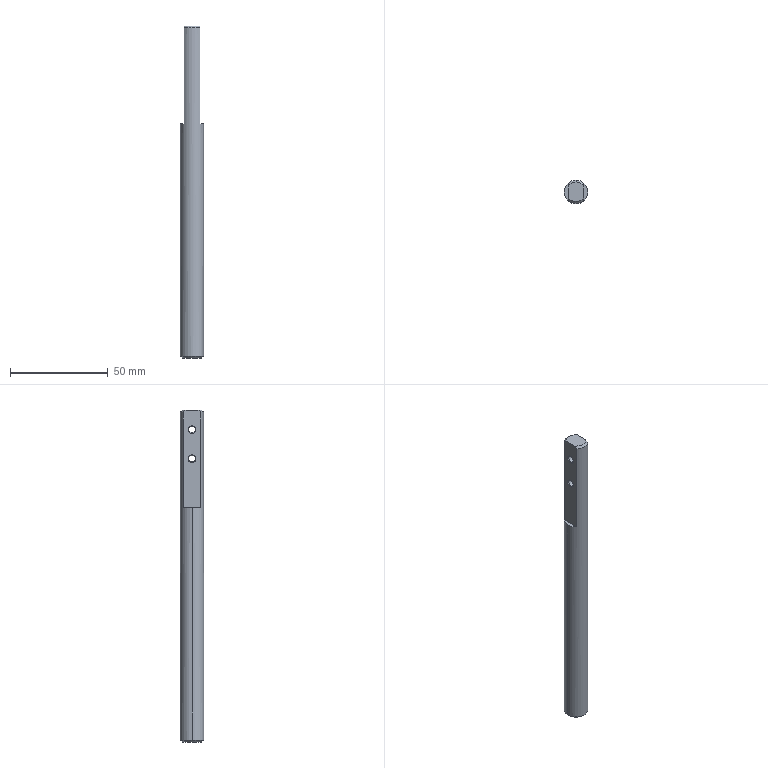Part | SolidWorks | features Chamfer 1, Extrusion 1, HoleWzd 1, ICE 1 | 1 solid | 20 faces | box 12 x 12 x 170 mm | volume 17822 mm3 | cone 8 | cylinder 6 | plane 6 | commonest cylinder face diameters 3.3 x4 12 x2
STEP:
#1=CARTESIAN_POINT('',(-3.625,0.,158.35));
#2=VERTEX_POINT('',#1);
#3=CARTESIAN_POINT('',(-3.625,0.,161.65));
#4=VERTEX_POINT('',#3);
#5=CARTESIAN_POINT('',(-3.625,0.,160.));
#6=DIRECTION('',(-1.,0.,0.));
#7=DIRECTION('',(0.,0.,1.));
#8=AXIS2_PLACEMENT_3D('',#5,#6,#7);
#9=CIRCLE('',#8,1.65);
#10=EDGE_CURVE('',#2,#4,#9,.T.);
#11=ORIENTED_EDGE('',*,*,#10,.F.);
#12=CARTESIAN_POINT('',(-4.,0.,157.975));
#13=VERTEX_POINT('',#12);
#14=CARTESIAN_POINT('',(-4.,0.,157.975));
#15=DIRECTION('',(-0.7071,0.,-0.7071));
#16=VECTOR('',#15,1000.);
#17=LINE('',#14,#16);
#18=EDGE_CURVE('',#2,#13,#17,.T.);
#19=ORIENTED_EDGE('',*,*,#18,.T.);
#20=CARTESIAN_POINT('',(-4.,0.,162.025));
#21=VERTEX_POINT('',#20);
#22=CARTESIAN_POINT('',(-4.,0.,160.));
#23=DIRECTION('',(-1.,0.,0.));
#24=DIRECTION('',(0.,0.,1.));
#25=AXIS2_PLACEMENT_3D('',#22,#23,#24);
#26=CIRCLE('',#25,2.025);
#27=EDGE_CURVE('',#13,#21,#26,.T.);
#28=ORIENTED_EDGE('',*,*,#27,.T.);
#29=CARTESIAN_POINT('',(-4.,0.,162.025));
#30=DIRECTION('',(-0.7071,0.,0.7071));
#31=VECTOR('',#30,1000.);
#32=LINE('',#29,#31);
#33=EDGE_CURVE('',#4,#21,#32,.T.);
#34=ORIENTED_EDGE('',*,*,#33,.F.);
#35=EDGE_LOOP('',(#11,#19,#28,#34));
#36=FACE_OUTER_BOUND('',#35,.T.);
#37=CARTESIAN_POINT('',(-4.,0.,160.));
#38=DIRECTION('',(-1.,0.,0.));
#39=DIRECTION('',(0.,0.,1.));
#40=AXIS2_PLACEMENT_3D('',#37,#38,#39);
#41=CONICAL_SURFACE('',#40,2.025,0.7854);
#42=ADVANCED_FACE('',(#36),#41,.F.);
#43=CARTESIAN_POINT('',(4.,0.,158.35));
#44=VERTEX_POINT('',#43);
#45=CARTESIAN_POINT('',(4.,0.,161.65));
#46=VERTEX_POINT('',#45);
#47=CARTESIAN_POINT('',(4.,0.,160.));
#48=DIRECTION('',(-1.,0.,0.));
#49=DIRECTION('',(0.,0.,1.));
#50=AXIS2_PLACEMENT_3D('',#47,#48,#49);
#51=CIRCLE('',#50,1.65);
#52=EDGE_CURVE('',#44,#46,#51,.T.);
#53=ORIENTED_EDGE('',*,*,#52,.F.);
#54=CARTESIAN_POINT('',(-4.,0.,158.35));
#55=DIRECTION('',(-1.,0.,0.));
#56=VECTOR('',#55,1000.);
#57=LINE('',#54,#56);
#58=EDGE_CURVE('',#44,#2,#57,.T.);
#59=ORIENTED_EDGE('',*,*,#58,.T.);
#60=ORIENTED_EDGE('',*,*,#10,.T.);
#61=CARTESIAN_POINT('',(-4.,0.,161.65));
#62=DIRECTION('',(-1.,0.,0.));
#63=VECTOR('',#62,1000.);
#64=LINE('',#61,#63);
#65=EDGE_CURVE('',#46,#4,#64,.T.);
#66=ORIENTED_EDGE('',*,*,#65,.F.);
#67=EDGE_LOOP('',(#53,#59,#60,#66));
#68=FACE_OUTER_BOUND('',#67,.T.);
#69=CARTESIAN_POINT('',(-4.,0.,160.));
#70=DIRECTION('',(-1.,0.,0.));
#71=DIRECTION('',(0.,0.,1.));
#72=AXIS2_PLACEMENT_3D('',#69,#70,#71);
#73=CYLINDRICAL_SURFACE('',#72,1.65);
#74=ADVANCED_FACE('',(#68),#73,.F.);
#75=CARTESIAN_POINT('',(-3.625,0.,143.35));
#76=VERTEX_POINT('',#75);
#77=CARTESIAN_POINT('',(-3.625,0.,146.65));
#78=VERTEX_POINT('',#77);
#79=CARTESIAN_POINT('',(-3.625,0.,145.));
#80=DIRECTION('',(-1.,0.,0.));
#81=DIRECTION('',(0.,0.,1.));
#82=AXIS2_PLACEMENT_3D('',#79,#80,#81);
#83=CIRCLE('',#82,1.65);
#84=EDGE_CURVE('',#76,#78,#83,.T.);
#85=ORIENTED_EDGE('',*,*,#84,.F.);
#86=CARTESIAN_POINT('',(-4.,0.,142.975));
#87=VERTEX_POINT('',#86);
#88=CARTESIAN_POINT('',(-4.,0.,142.975));
#89=DIRECTION('',(-0.7071,0.,-0.7071));
#90=VECTOR('',#89,1000.);
#91=LINE('',#88,#90);
#92=EDGE_CURVE('',#76,#87,#91,.T.);
#93=ORIENTED_EDGE('',*,*,#92,.T.);
#94=CARTESIAN_POINT('',(-4.,0.,147.025));
#95=VERTEX_POINT('',#94);
#96=CARTESIAN_POINT('',(-4.,0.,145.));
#97=DIRECTION('',(-1.,0.,0.));
#98=DIRECTION('',(0.,0.,1.));
#99=AXIS2_PLACEMENT_3D('',#96,#97,#98);
#100=CIRCLE('',#99,2.025);
#101=EDGE_CURVE('',#87,#95,#100,.T.);
#102=ORIENTED_EDGE('',*,*,#101,.T.);
#103=CARTESIAN_POINT('',(-4.,0.,147.025));
#104=DIRECTION('',(-0.7071,0.,0.7071));
#105=VECTOR('',#104,1000.);
#106=LINE('',#103,#105);
#107=EDGE_CURVE('',#78,#95,#106,.T.);
#108=ORIENTED_EDGE('',*,*,#107,.F.);
#109=EDGE_LOOP('',(#85,#93,#102,#108));
#110=FACE_OUTER_BOUND('',#109,.T.);
#111=CARTESIAN_POINT('',(-4.,0.,145.));
#112=DIRECTION('',(-1.,0.,0.));
#113=DIRECTION('',(0.,0.,1.));
#114=AXIS2_PLACEMENT_3D('',#111,#112,#113);
#115=CONICAL_SURFACE('',#114,2.025,0.7854);
#116=ADVANCED_FACE('',(#110),#115,.F.);
#117=CARTESIAN_POINT('',(4.,0.,143.35));
#118=VERTEX_POINT('',#117);
#119=CARTESIAN_POINT('',(4.,0.,146.65));
#120=VERTEX_POINT('',#119);
#121=CARTESIAN_POINT('',(4.,0.,145.));
#122=DIRECTION('',(-1.,0.,0.));
#123=DIRECTION('',(0.,0.,1.));
#124=AXIS2_PLACEMENT_3D('',#121,#122,#123);
#125=CIRCLE('',#124,1.65);
#126=EDGE_CURVE('',#118,#120,#125,.T.);
#127=ORIENTED_EDGE('',*,*,#126,.F.);
#128=CARTESIAN_POINT('',(-4.,0.,143.35));
#129=DIRECTION('',(-1.,0.,0.));
#130=VECTOR('',#129,1000.);
#131=LINE('',#128,#130);
#132=EDGE_CURVE('',#118,#76,#131,.T.);
#133=ORIENTED_EDGE('',*,*,#132,.T.);
#134=ORIENTED_EDGE('',*,*,#84,.T.);
#135=CARTESIAN_POINT('',(-4.,0.,146.65));
#136=DIRECTION('',(-1.,0.,0.));
#137=VECTOR('',#136,1000.);
#138=LINE('',#135,#137);
#139=EDGE_CURVE('',#120,#78,#138,.T.);
#140=ORIENTED_EDGE('',*,*,#139,.F.);
#141=EDGE_LOOP('',(#127,#133,#134,#140));
#142=FACE_OUTER_BOUND('',#141,.T.);
#143=CARTESIAN_POINT('',(-4.,0.,145.));
#144=DIRECTION('',(-1.,0.,0.));
#145=DIRECTION('',(0.,0.,1.));
#146=AXIS2_PLACEMENT_3D('',#143,#144,#145);
#147=CYLINDRICAL_SURFACE('',#146,1.65);
#148=ADVANCED_FACE('',(#142),#147,.F.);
#149=CARTESIAN_POINT('',(-5.,0.,0.));
#150=VERTEX_POINT('',#149);
#151=CARTESIAN_POINT('',(5.,0.,0.));
#152=VERTEX_POINT('',#151);
#153=CARTESIAN_POINT('',(0.,0.,0.));
#154=DIRECTION('',(0.,0.,-1.));
#155=DIRECTION('',(1.,0.,0.));
#156=AXIS2_PLACEMENT_3D('',#153,#154,#155);
#157=CIRCLE('',#156,5.);
#158=EDGE_CURVE('',#150,#152,#157,.T.);
#159=ORIENTED_EDGE('',*,*,#158,.F.);
#160=CARTESIAN_POINT('',(-6.,0.,1.));
#161=VERTEX_POINT('',#160);
#162=CARTESIAN_POINT('',(-6.,0.,1.));
#163=DIRECTION('',(-0.7071,0.,0.7071));
#164=VECTOR('',#163,1000.);
#165=LINE('',#162,#164);
#166=EDGE_CURVE('',#150,#161,#165,.T.);
#167=ORIENTED_EDGE('',*,*,#166,.T.);
#168=CARTESIAN_POINT('',(6.,0.,1.));
#169=VERTEX_POINT('',#168);
#170=CARTESIAN_POINT('',(0.,0.,1.));
#171=DIRECTION('',(0.,0.,1.));
#172=DIRECTION('',(1.,0.,0.));
#173=AXIS2_PLACEMENT_3D('',#170,#171,#172);
#174=CIRCLE('',#173,6.);
#175=EDGE_CURVE('',#169,#161,#174,.T.);
#176=ORIENTED_EDGE('',*,*,#175,.F.);
#177=CARTESIAN_POINT('',(6.,0.,1.));
#178=DIRECTION('',(0.7071,0.,0.7071));
#179=VECTOR('',#178,1000.);
#180=LINE('',#177,#179);
#181=EDGE_CURVE('',#152,#169,#180,.T.);
#182=ORIENTED_EDGE('',*,*,#181,.F.);
#183=EDGE_LOOP('',(#159,#167,#176,#182));
#184=FACE_OUTER_BOUND('',#183,.T.);
#185=CARTESIAN_POINT('',(0.,0.,1.));
#186=DIRECTION('',(0.,0.,1.));
#187=DIRECTION('',(1.,0.,0.));
#188=AXIS2_PLACEMENT_3D('',#185,#186,#187);
#189=CONICAL_SURFACE('',#188,6.,0.7854);
#190=ADVANCED_FACE('',(#184),#189,.T.);
#191=CARTESIAN_POINT('',(4.,4.472,120.));
#192=VERTEX_POINT('',#191);
#193=CARTESIAN_POINT('',(6.,0.,120.));
#194=VERTEX_POINT('',#193);
#195=CARTESIAN_POINT('',(0.,0.,120.));
#196=DIRECTION('',(0.,0.,-1.));
#197=DIRECTION('',(-1.,0.,0.));
#198=AXIS2_PLACEMENT_3D('',#195,#196,#197);
#199=CIRCLE('',#198,6.);
#200=EDGE_CURVE('',#192,#194,#199,.T.);
#201=ORIENTED_EDGE('',*,*,#200,.T.);
#202=CARTESIAN_POINT('',(6.,0.,170.));
#203=DIRECTION('',(0.,0.,-1.));
#204=VECTOR('',#203,1000.);
#205=LINE('',#202,#204);
#206=EDGE_CURVE('',#194,#169,#205,.T.);
#207=ORIENTED_EDGE('',*,*,#206,.T.);
#208=ORIENTED_EDGE('',*,*,#175,.T.);
#209=CARTESIAN_POINT('',(-6.,0.,120.));
#210=VERTEX_POINT('',#209);
#211=CARTESIAN_POINT('',(-6.,0.,170.));
#212=DIRECTION('',(0.,0.,-1.));
#213=VECTOR('',#212,1000.);
#214=LINE('',#211,#213);
#215=EDGE_CURVE('',#210,#161,#214,.T.);
#216=ORIENTED_EDGE('',*,*,#215,.F.);
#217=CARTESIAN_POINT('',(-4.,4.472,120.));
#218=VERTEX_POINT('',#217);
#219=CARTESIAN_POINT('',(0.,0.,120.));
#220=DIRECTION('',(0.,0.,-1.));
#221=DIRECTION('',(-1.,0.,0.));
#222=AXIS2_PLACEMENT_3D('',#219,#220,#221);
#223=CIRCLE('',#222,6.);
#224=EDGE_CURVE('',#210,#218,#223,.T.);
#225=ORIENTED_EDGE('',*,*,#224,.T.);
#226=CARTESIAN_POINT('',(-4.,4.472,169.));
#227=VERTEX_POINT('',#226);
#228=CARTESIAN_POINT('',(-4.,4.472,170.));
#229=DIRECTION('',(0.,0.,1.));
#230=VECTOR('',#229,1000.);
#231=LINE('',#228,#230);
#232=EDGE_CURVE('',#218,#227,#231,.T.);
#233=ORIENTED_EDGE('',*,*,#232,.T.);
#234=CARTESIAN_POINT('',(4.,4.472,169.));
#235=VERTEX_POINT('',#234);
#236=CARTESIAN_POINT('',(0.,0.,169.));
#237=DIRECTION('',(0.,0.,-1.));
#238=DIRECTION('',(1.,0.,0.));
#239=AXIS2_PLACEMENT_3D('',#236,#237,#238);
#240=CIRCLE('',#239,6.);
#241=EDGE_CURVE('',#227,#235,#240,.T.);
#242=ORIENTED_EDGE('',*,*,#241,.T.);
#243=CARTESIAN_POINT('',(4.,4.472,170.));
#244=DIRECTION('',(0.,0.,-1.));
#245=VECTOR('',#244,1000.);
#246=LINE('',#243,#245);
#247=EDGE_CURVE('',#235,#192,#246,.T.);
#248=ORIENTED_EDGE('',*,*,#247,.T.);
#249=EDGE_LOOP('',(#201,#207,#208,#216,#225,#233,#242,#248));
#250=FACE_OUTER_BOUND('',#249,.T.);
#251=CARTESIAN_POINT('',(0.,0.,170.));
#252=DIRECTION('',(0.,0.,-1.));
#253=DIRECTION('',(-1.,0.,0.));
#254=AXIS2_PLACEMENT_3D('',#251,#252,#253);
#255=CYLINDRICAL_SURFACE('',#254,6.);
#256=ADVANCED_FACE('',(#250),#255,.T.);
#257=CARTESIAN_POINT('',(-4.,0.,160.));
#258=DIRECTION('',(-1.,0.,0.));
#259=DIRECTION('',(0.,0.,1.));
#260=AXIS2_PLACEMENT_3D('',#257,#258,#259);
#261=CIRCLE('',#260,2.025);
#262=EDGE_CURVE('',#21,#13,#261,.T.);
#263=ORIENTED_EDGE('',*,*,#262,.F.);
#264=ORIENTED_EDGE('',*,*,#27,.F.);
#265=EDGE_LOOP('',(#263,#264));
#266=FACE_BOUND('',#265,.T.);
#267=CARTESIAN_POINT('',(-4.,-4.472,169.));
#268=VERTEX_POINT('',#267);
#269=CARTESIAN_POINT('',(-4.,-3.,170.));
#270=VERTEX_POINT('',#269);
#271=CARTESIAN_POINT('',(-4.,-4.472,169.));
#272=CARTESIAN_POINT('',(-4.,-3.994,169.356));
#273=CARTESIAN_POINT('',(-4.,-3.507,169.696));
#274=CARTESIAN_POINT('',(-4.,-3.,170.));
#275=B_SPLINE_CURVE_WITH_KNOTS('',3,(#271,#272,#273,#274),.UNSPECIFIED.,.F.,.F.,(4,4),(0.000001163,0.001776),.UNSPECIFIED.);
#276=EDGE_CURVE('',#268,#270,#275,.T.);
#277=ORIENTED_EDGE('',*,*,#276,.T.);
#278=CARTESIAN_POINT('',(-4.,3.,170.));
#279=VERTEX_POINT('',#278);
#280=CARTESIAN_POINT('',(-4.,-6.,170.));
#281=DIRECTION('',(0.,1.,0.));
#282=VECTOR('',#281,1000.);
#283=LINE('',#280,#282);
#284=EDGE_CURVE('',#270,#279,#283,.T.);
#285=ORIENTED_EDGE('',*,*,#284,.T.);
#286=CARTESIAN_POINT('',(-4.,3.,170.));
#287=CARTESIAN_POINT('',(-4.,3.508,169.695));
#288=CARTESIAN_POINT('',(-4.,3.995,169.356));
#289=CARTESIAN_POINT('',(-4.,4.472,169.));
#290=B_SPLINE_CURVE_WITH_KNOTS('',3,(#286,#287,#288,#289),.UNSPECIFIED.,.F.,.F.,(4,4),(0.008119,0.009881),.UNSPECIFIED.);
#291=EDGE_CURVE('',#279,#227,#290,.T.);
#292=ORIENTED_EDGE('',*,*,#291,.T.);
#293=ORIENTED_EDGE('',*,*,#232,.F.);
#294=CARTESIAN_POINT('',(-4.,-4.472,120.));
#295=VERTEX_POINT('',#294);
#296=CARTESIAN_POINT('',(-4.,-6.,120.));
#297=DIRECTION('',(0.,1.,0.));
#298=VECTOR('',#297,1000.);
#299=LINE('',#296,#298);
#300=EDGE_CURVE('',#295,#218,#299,.T.);
#301=ORIENTED_EDGE('',*,*,#300,.F.);
#302=CARTESIAN_POINT('',(-4.,-4.472,170.));
#303=DIRECTION('',(0.,0.,-1.));
#304=VECTOR('',#303,1000.);
#305=LINE('',#302,#304);
#306=EDGE_CURVE('',#268,#295,#305,.T.);
#307=ORIENTED_EDGE('',*,*,#306,.F.);
#308=EDGE_LOOP('',(#277,#285,#292,#293,#301,#307));
#309=FACE_OUTER_BOUND('',#308,.T.);
#310=CARTESIAN_POINT('',(-4.,0.,145.));
#311=DIRECTION('',(-1.,0.,0.));
#312=DIRECTION('',(0.,0.,1.));
#313=AXIS2_PLACEMENT_3D('',#310,#311,#312);
#314=CIRCLE('',#313,2.025);
#315=EDGE_CURVE('',#95,#87,#314,.T.);
#316=ORIENTED_EDGE('',*,*,#315,.F.);
#317=ORIENTED_EDGE('',*,*,#101,.F.);
#318=EDGE_LOOP('',(#316,#317));
#319=FACE_BOUND('',#318,.T.);
#320=CARTESIAN_POINT('',(-4.,-6.,120.));
#321=DIRECTION('',(1.,0.,0.));
#322=DIRECTION('',(0.,0.,-1.));
#323=AXIS2_PLACEMENT_3D('',#320,#321,#322);
#324=PLANE('',#323);
#325=ADVANCED_FACE('',(#266,#309,#319),#324,.F.);
#326=ORIENTED_EDGE('',*,*,#276,.F.);
#327=CARTESIAN_POINT('',(4.,-4.472,169.));
#328=VERTEX_POINT('',#327);
#329=CARTESIAN_POINT('',(0.,0.,169.));
#330=DIRECTION('',(0.,0.,-1.));
#331=DIRECTION('',(1.,0.,0.));
#332=AXIS2_PLACEMENT_3D('',#329,#330,#331);
#333=CIRCLE('',#332,6.);
#334=EDGE_CURVE('',#328,#268,#333,.T.);
#335=ORIENTED_EDGE('',*,*,#334,.F.);
#336=CARTESIAN_POINT('',(4.,-3.,170.));
#337=VERTEX_POINT('',#336);
#338=CARTESIAN_POINT('',(4.,-3.,170.));
#339=CARTESIAN_POINT('',(4.,-3.508,169.695));
#340=CARTESIAN_POINT('',(4.,-3.995,169.356));
#341=CARTESIAN_POINT('',(4.,-4.472,169.));
#342=B_SPLINE_CURVE_WITH_KNOTS('',3,(#338,#339,#340,#341),.UNSPECIFIED.,.F.,.F.,(4,4),(0.008119,0.009881),.UNSPECIFIED.);
#343=EDGE_CURVE('',#337,#328,#342,.T.);
#344=ORIENTED_EDGE('',*,*,#343,.F.);
#345=CARTESIAN_POINT('',(0.,0.,170.));
#346=DIRECTION('',(0.,0.,1.));
#347=DIRECTION('',(1.,0.,0.));
#348=AXIS2_PLACEMENT_3D('',#345,#346,#347);
#349=CIRCLE('',#348,5.);
#350=EDGE_CURVE('',#270,#337,#349,.T.);
#351=ORIENTED_EDGE('',*,*,#350,.F.);
#352=EDGE_LOOP('',(#326,#335,#344,#351));
#353=FACE_OUTER_BOUND('',#352,.T.);
#354=CARTESIAN_POINT('',(0.,0.,170.));
#355=DIRECTION('',(0.,0.,-1.));
#356=DIRECTION('',(-1.,0.,0.));
#357=AXIS2_PLACEMENT_3D('',#354,#355,#356);
#358=CONICAL_SURFACE('',#357,5.,0.7854);
#359=ADVANCED_FACE('',(#353),#358,.T.);
#360=ORIENTED_EDGE('',*,*,#206,.F.);
#361=CARTESIAN_POINT('',(4.,-4.472,120.));
#362=VERTEX_POINT('',#361);
#363=CARTESIAN_POINT('',(0.,0.,120.));
#364=DIRECTION('',(0.,0.,-1.));
#365=DIRECTION('',(-1.,0.,0.));
#366=AXIS2_PLACEMENT_3D('',#363,#364,#365);
#367=CIRCLE('',#366,6.);
#368=EDGE_CURVE('',#194,#362,#367,.T.);
#369=ORIENTED_EDGE('',*,*,#368,.T.);
#370=CARTESIAN_POINT('',(4.,-4.472,170.));
#371=DIRECTION('',(0.,0.,1.));
#372=VECTOR('',#371,1000.);
#373=LINE('',#370,#372);
#374=EDGE_CURVE('',#362,#328,#373,.T.);
#375=ORIENTED_EDGE('',*,*,#374,.T.);
#376=ORIENTED_EDGE('',*,*,#334,.T.);
#377=ORIENTED_EDGE('',*,*,#306,.T.);
#378=CARTESIAN_POINT('',(0.,0.,120.));
#379=DIRECTION('',(0.,0.,-1.));
#380=DIRECTION('',(-1.,0.,0.));
#381=AXIS2_PLACEMENT_3D('',#378,#379,#380);
#382=CIRCLE('',#381,6.);
#383=EDGE_CURVE('',#295,#210,#382,.T.);
#384=ORIENTED_EDGE('',*,*,#383,.T.);
#385=ORIENTED_EDGE('',*,*,#215,.T.);
#386=CARTESIAN_POINT('',(0.,0.,1.));
#387=DIRECTION('',(0.,0.,1.));
#388=DIRECTION('',(1.,0.,0.));
#389=AXIS2_PLACEMENT_3D('',#386,#387,#388);
#390=CIRCLE('',#389,6.);
#391=EDGE_CURVE('',#161,#169,#390,.T.);
#392=ORIENTED_EDGE('',*,*,#391,.T.);
#393=EDGE_LOOP('',(#360,#369,#375,#376,#377,#384,#385,#392));
#394=FACE_OUTER_BOUND('',#393,.T.);
#395=CARTESIAN_POINT('',(0.,0.,170.));
#396=DIRECTION('',(0.,0.,-1.));
#397=DIRECTION('',(-1.,0.,0.));
#398=AXIS2_PLACEMENT_3D('',#395,#396,#397);
#399=CYLINDRICAL_SURFACE('',#398,6.);
#400=ADVANCED_FACE('',(#394),#399,.T.);
#401=ORIENTED_EDGE('',*,*,#284,.F.);
#402=ORIENTED_EDGE('',*,*,#350,.T.);
#403=CARTESIAN_POINT('',(4.,3.,170.));
#404=VERTEX_POINT('',#403);
#405=CARTESIAN_POINT('',(4.,-6.,170.));
#406=DIRECTION('',(0.,1.,0.));
#407=VECTOR('',#406,1000.);
#408=LINE('',#405,#407);
#409=EDGE_CURVE('',#337,#404,#408,.T.);
#410=ORIENTED_EDGE('',*,*,#409,.T.);
#411=CARTESIAN_POINT('',(0.,0.,170.));
#412=DIRECTION('',(0.,0.,1.));
#413=DIRECTION('',(1.,0.,0.));
#414=AXIS2_PLACEMENT_3D('',#411,#412,#413);
#415=CIRCLE('',#414,5.);
#416=EDGE_CURVE('',#404,#279,#415,.T.);
#417=ORIENTED_EDGE('',*,*,#416,.T.);
#418=EDGE_LOOP('',(#401,#402,#410,#417));
#419=FACE_OUTER_BOUND('',#418,.T.);
#420=CARTESIAN_POINT('',(0.,0.,170.));
#421=DIRECTION('',(0.,0.,1.));
#422=DIRECTION('',(1.,0.,0.));
#423=AXIS2_PLACEMENT_3D('',#420,#421,#422);
#424=PLANE('',#423);
#425=ADVANCED_FACE('',(#419),#424,.T.);
#426=CARTESIAN_POINT('',(0.,0.,0.));
#427=DIRECTION('',(0.,0.,-1.));
#428=DIRECTION('',(1.,0.,0.));
#429=AXIS2_PLACEMENT_3D('',#426,#427,#428);
#430=CIRCLE('',#429,5.);
#431=EDGE_CURVE('',#152,#150,#430,.T.);
#432=ORIENTED_EDGE('',*,*,#431,.T.);
#433=ORIENTED_EDGE('',*,*,#158,.T.);
#434=EDGE_LOOP('',(#432,#433));
#435=FACE_OUTER_BOUND('',#434,.T.);
#436=CARTESIAN_POINT('',(0.,0.,0.));
#437=DIRECTION('',(0.,0.,1.));
#438=DIRECTION('',(1.,0.,0.));
#439=AXIS2_PLACEMENT_3D('',#436,#437,#438);
#440=PLANE('',#439);
#441=ADVANCED_FACE('',(#435),#440,.F.);
#442=ORIENTED_EDGE('',*,*,#291,.F.);
#443=ORIENTED_EDGE('',*,*,#416,.F.);
#444=CARTESIAN_POINT('',(4.,4.472,169.));
#445=CARTESIAN_POINT('',(4.,3.994,169.356));
#446=CARTESIAN_POINT('',(4.,3.507,169.696));
#447=CARTESIAN_POINT('',(4.,3.,170.));
#448=B_SPLINE_CURVE_WITH_KNOTS('',3,(#444,#445,#446,#447),.UNSPECIFIED.,.F.,.F.,(4,4),(0.000001163,0.001776),.UNSPECIFIED.);
#449=EDGE_CURVE('',#235,#404,#448,.T.);
#450=ORIENTED_EDGE('',*,*,#449,.F.);
#451=ORIENTED_EDGE('',*,*,#241,.F.);
#452=EDGE_LOOP('',(#442,#443,#450,#451));
#453=FACE_OUTER_BOUND('',#452,.T.);
#454=CARTESIAN_POINT('',(0.,0.,170.));
#455=DIRECTION('',(0.,0.,-1.));
#456=DIRECTION('',(-1.,0.,0.));
#457=AXIS2_PLACEMENT_3D('',#454,#455,#456);
#458=CONICAL_SURFACE('',#457,5.,0.7854);
#459=ADVANCED_FACE('',(#453),#458,.T.);
#460=ORIENTED_EDGE('',*,*,#166,.F.);
#461=ORIENTED_EDGE('',*,*,#431,.F.);
#462=ORIENTED_EDGE('',*,*,#181,.T.);
#463=ORIENTED_EDGE('',*,*,#391,.F.);
#464=EDGE_LOOP('',(#460,#461,#462,#463));
#465=FACE_OUTER_BOUND('',#464,.T.);
#466=CARTESIAN_POINT('',(0.,0.,1.));
#467=DIRECTION('',(0.,0.,1.));
#468=DIRECTION('',(1.,0.,0.));
#469=AXIS2_PLACEMENT_3D('',#466,#467,#468);
#470=CONICAL_SURFACE('',#469,6.,0.7854);
#471=ADVANCED_FACE('',(#465),#470,.T.);
#472=CARTESIAN_POINT('',(4.,-6.,120.));
#473=DIRECTION('',(0.,1.,0.));
#474=VECTOR('',#473,1000.);
#475=LINE('',#472,#474);
#476=EDGE_CURVE('',#362,#192,#475,.T.);
#477=ORIENTED_EDGE('',*,*,#476,.F.);
#478=ORIENTED_EDGE('',*,*,#368,.F.);
#479=ORIENTED_EDGE('',*,*,#200,.F.);
#480=EDGE_LOOP('',(#477,#478,#479));
#481=FACE_OUTER_BOUND('',#480,.T.);
#482=CARTESIAN_POINT('',(6.,-6.,120.));
#483=DIRECTION('',(0.,0.,-1.));
#484=DIRECTION('',(-1.,0.,0.));
#485=AXIS2_PLACEMENT_3D('',#482,#483,#484);
#486=PLANE('',#485);
#487=ADVANCED_FACE('',(#481),#486,.F.);
#488=CARTESIAN_POINT('',(4.,0.,160.));
#489=DIRECTION('',(-1.,0.,0.));
#490=DIRECTION('',(0.,0.,1.));
#491=AXIS2_PLACEMENT_3D('',#488,#489,#490);
#492=CIRCLE('',#491,1.65);
#493=EDGE_CURVE('',#46,#44,#492,.T.);
#494=ORIENTED_EDGE('',*,*,#493,.T.);
#495=ORIENTED_EDGE('',*,*,#52,.T.);
#496=EDGE_LOOP('',(#494,#495));
#497=FACE_BOUND('',#496,.T.);
#498=CARTESIAN_POINT('',(4.,0.,145.));
#499=DIRECTION('',(-1.,0.,0.));
#500=DIRECTION('',(0.,0.,1.));
#501=AXIS2_PLACEMENT_3D('',#498,#499,#500);
#502=CIRCLE('',#501,1.65);
#503=EDGE_CURVE('',#120,#118,#502,.T.);
#504=ORIENTED_EDGE('',*,*,#503,.T.);
#505=ORIENTED_EDGE('',*,*,#126,.T.);
#506=EDGE_LOOP('',(#504,#505));
#507=FACE_BOUND('',#506,.T.);
#508=ORIENTED_EDGE('',*,*,#449,.T.);
#509=ORIENTED_EDGE('',*,*,#409,.F.);
#510=ORIENTED_EDGE('',*,*,#343,.T.);
#511=ORIENTED_EDGE('',*,*,#374,.F.);
#512=ORIENTED_EDGE('',*,*,#476,.T.);
#513=ORIENTED_EDGE('',*,*,#247,.F.);
#514=EDGE_LOOP('',(#508,#509,#510,#511,#512,#513));
#515=FACE_OUTER_BOUND('',#514,.T.);
#516=CARTESIAN_POINT('',(4.,-6.,120.));
#517=DIRECTION('',(-1.,0.,0.));
#518=DIRECTION('',(0.,0.,1.));
#519=AXIS2_PLACEMENT_3D('',#516,#517,#518);
#520=PLANE('',#519);
#521=ADVANCED_FACE('',(#497,#507,#515),#520,.F.);
#522=ORIENTED_EDGE('',*,*,#383,.F.);
#523=ORIENTED_EDGE('',*,*,#300,.T.);
#524=ORIENTED_EDGE('',*,*,#224,.F.);
#525=EDGE_LOOP('',(#522,#523,#524));
#526=FACE_OUTER_BOUND('',#525,.T.);
#527=CARTESIAN_POINT('',(-6.,-6.,120.));
#528=DIRECTION('',(0.,0.,-1.));
#529=DIRECTION('',(-1.,0.,0.));
#530=AXIS2_PLACEMENT_3D('',#527,#528,#529);
#531=PLANE('',#530);
#532=ADVANCED_FACE('',(#526),#531,.F.);
#533=ORIENTED_EDGE('',*,*,#132,.F.);
#534=ORIENTED_EDGE('',*,*,#503,.F.);
#535=ORIENTED_EDGE('',*,*,#139,.T.);
#536=CARTESIAN_POINT('',(-3.625,0.,145.));
#537=DIRECTION('',(-1.,0.,0.));
#538=DIRECTION('',(0.,0.,1.));
#539=AXIS2_PLACEMENT_3D('',#536,#537,#538);
#540=CIRCLE('',#539,1.65);
#541=EDGE_CURVE('',#78,#76,#540,.T.);
#542=ORIENTED_EDGE('',*,*,#541,.T.);
#543=EDGE_LOOP('',(#533,#534,#535,#542));
#544=FACE_OUTER_BOUND('',#543,.T.);
#545=CARTESIAN_POINT('',(-4.,0.,145.));
#546=DIRECTION('',(-1.,0.,0.));
#547=DIRECTION('',(0.,0.,1.));
#548=AXIS2_PLACEMENT_3D('',#545,#546,#547);
#549=CYLINDRICAL_SURFACE('',#548,1.65);
#550=ADVANCED_FACE('',(#544),#549,.F.);
#551=ORIENTED_EDGE('',*,*,#92,.F.);
#552=ORIENTED_EDGE('',*,*,#541,.F.);
#553=ORIENTED_EDGE('',*,*,#107,.T.);
#554=ORIENTED_EDGE('',*,*,#315,.T.);
#555=EDGE_LOOP('',(#551,#552,#553,#554));
#556=FACE_OUTER_BOUND('',#555,.T.);
#557=CARTESIAN_POINT('',(-4.,0.,145.));
#558=DIRECTION('',(-1.,0.,0.));
#559=DIRECTION('',(0.,0.,1.));
#560=AXIS2_PLACEMENT_3D('',#557,#558,#559);
#561=CONICAL_SURFACE('',#560,2.025,0.7854);
#562=ADVANCED_FACE('',(#556),#561,.F.);
#563=ORIENTED_EDGE('',*,*,#58,.F.);
#564=ORIENTED_EDGE('',*,*,#493,.F.);
#565=ORIENTED_EDGE('',*,*,#65,.T.);
#566=CARTESIAN_POINT('',(-3.625,0.,160.));
#567=DIRECTION('',(-1.,0.,0.));
#568=DIRECTION('',(0.,0.,1.));
#569=AXIS2_PLACEMENT_3D('',#566,#567,#568);
#570=CIRCLE('',#569,1.65);
#571=EDGE_CURVE('',#4,#2,#570,.T.);
#572=ORIENTED_EDGE('',*,*,#571,.T.);
#573=EDGE_LOOP('',(#563,#564,#565,#572));
#574=FACE_OUTER_BOUND('',#573,.T.);
#575=CARTESIAN_POINT('',(-4.,0.,160.));
#576=DIRECTION('',(-1.,0.,0.));
#577=DIRECTION('',(0.,0.,1.));
#578=AXIS2_PLACEMENT_3D('',#575,#576,#577);
#579=CYLINDRICAL_SURFACE('',#578,1.65);
#580=ADVANCED_FACE('',(#574),#579,.F.);
#581=ORIENTED_EDGE('',*,*,#18,.F.);
#582=ORIENTED_EDGE('',*,*,#571,.F.);
#583=ORIENTED_EDGE('',*,*,#33,.T.);
#584=ORIENTED_EDGE('',*,*,#262,.T.);
#585=EDGE_LOOP('',(#581,#582,#583,#584));
#586=FACE_OUTER_BOUND('',#585,.T.);
#587=CARTESIAN_POINT('',(-4.,0.,160.));
#588=DIRECTION('',(-1.,0.,0.));
#589=DIRECTION('',(0.,0.,1.));
#590=AXIS2_PLACEMENT_3D('',#587,#588,#589);
#591=CONICAL_SURFACE('',#590,2.025,0.7854);
#592=ADVANCED_FACE('',(#586),#591,.F.);
#593=CLOSED_SHELL('',(#42,#74,#116,#148,#190,#256,#325,#359,#400,#425,#441,#459,#471,#487,#521,#532,#550,#562,#580,#592));
#594=MANIFOLD_SOLID_BREP('',#593);
#595=CARTESIAN_POINT('',(0.,0.,0.));
#596=DIRECTION('',(0.,0.,1.));
#597=DIRECTION('',(1.,0.,0.));
#598=AXIS2_PLACEMENT_3D('',#595,#596,#597);
#599=(LENGTH_UNIT()NAMED_UNIT(*)SI_UNIT(.MILLI.,.METRE.));
#600=UNCERTAINTY_MEASURE_WITH_UNIT(LENGTH_MEASURE(0.00001),#599,'','');
#601=(NAMED_UNIT(*)PLANE_ANGLE_UNIT()SI_UNIT($,.RADIAN.));
#602=(NAMED_UNIT(*)SI_UNIT($,.STERADIAN.)SOLID_ANGLE_UNIT());
#603=(GEOMETRIC_REPRESENTATION_CONTEXT(3)GLOBAL_UNCERTAINTY_ASSIGNED_CONTEXT((#600))GLOBAL_UNIT_ASSIGNED_CONTEXT((#599,#601,#602))REPRESENTATION_CONTEXT('',''));
#604=ADVANCED_BREP_SHAPE_REPRESENTATION('',(#594,#598),#603);